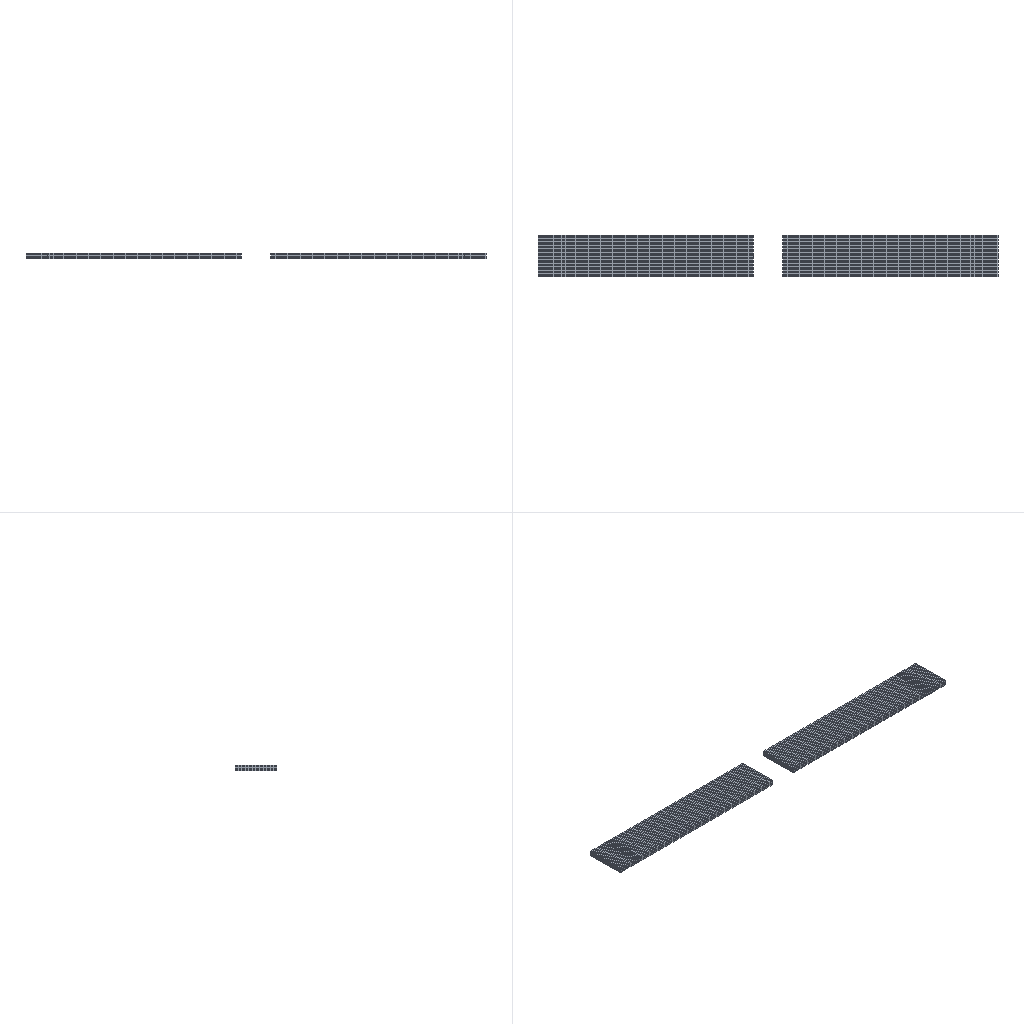Simulation study | abaqus
Set-up summary:
category,name,step,type,value,unit,region
solver,abaqus
solver,version,,,Abaqus/Standard 2020
units,not stated in the deck,,not stated
analysis,deck,,transient,transient
load_step,Step-1,Step-1,transient
load_step,requested,,,1
mesh,nodes,,,9920
mesh,elements,,,7200
element_type,C3D8R,,solid,7200
load,load commands in deck,,count,1
bc,support commands in deck,,count,6
material,MATERIAL-1,,in results
check,setup vs results,,match,"per instance, exact: element labels, types and connectivity; labels of the nodes the elements use; coordinates of those nodes at SINGLE_PRECISION in 1 of 4 instance(s)"
Abaqus input file, long lists of numbers shortened:
*Heading
** Job name: Job-1 Model name: Model-1
** Generated by: Abaqus/CAE 2020
*Preprint, echo=NO, model=NO, history=NO, contact=NO
**
** PARTS
**
*Part, name=Part-1
*Node
      1,           0.,           0.,           0.
      2,           0.,          -1.,           0.
** (4028 more lines like these left out)
*Element, type=C3D8R
   1,  156,  157,  188,  187,    1,    2,   33,   32
   2,  157,  158,  189,  188,    2,    3,   34,   33
** (2998 more lines like these left out)
*Nset, nset=Set-6, generate
    1,  4030,     1
*Elset, elset=Set-6, generate
    1,  3000,     1
** Section: Section-1
*Solid Section, elset=Set-6, material=Material-1
,
*End Part
**
*Part, name=Part-2
*Node
      1,           0.,         -30.,           4.
      2,           0.,         -29.,           4.
** (928 more lines like these left out)
*Element, type=C3D8R
  1, 156, 157, 188, 187,   1,   2,  33,  32
  2, 157, 158, 189, 188,   2,   3,  34,  33
** (598 more lines like these left out)
*Nset, nset=Set-7, generate
   1,  930,    1
*Elset, elset=Set-7, generate
   1,  600,    1
** Section: Section-1
*Solid Section, elset=Set-7, material=Material-1
,
*End Part
**
**
** ASSEMBLY
**
*Assembly, name=Assembly
**
*Instance, name=Part-1-1, part=Part-1
*End Instance
**
*Instance, name=Part-2-1, part=Part-2
       -15.5,           0.,           0.
*End Instance
**
*Instance, name=Part-1-1-rad-2, part=Part-1
        300.,         -30.,           0.
        300.,         -30.,           0.,         300.,         -30.,           1.,         180.
*End Instance
**
*Instance, name=Part-2-1-rad-2, part=Part-2
       315.5,         -30.,           0.
       315.5,         -30.,           0.,        315.5,         -30.,           1.,         180.
*End Instance
**
*Node
      1,         150.,         -15.,           2.
*Node
      2,         150.,         -15.,           3.
*Node
      3,         150.,         -15.,          2.5
*Node
      4,         150.,         -13.,          2.5
*Nset, nset=Set-2
 3,
*Nset, nset=Set-3, instance=Part-1-1
    1,   31,   94,  124,  125,  155,  931,  961, 1055, 1085, 3876, 3906, 4000, 4030
*Nset, nset=Set-3, instance=Part-2-1
   1,  31, 125, 155, 156, 186, 280, 310, 621, 651, 745, 775, 776, 806, 838, 868
 900, 930
*Nset, nset=Set-3, generate
 1,  3,  1
*Nset, nset=Set-3, instance=Part-1-1-rad-2
    1,   31,   94,  124,  125,  155,  931,  961, 1055, 1085, 3876, 3906, 4000, 4030
*Nset, nset=Set-3, instance=Part-2-1-rad-2
   1,  31, 125, 155, 156, 186, 280, 310, 621, 651, 745, 775, 776, 806, 838, 868
 900, 930
*Nset, nset=Set-4, instance=Part-1-1, generate
    1,  4030,     1
*Nset, nset=Set-4, instance=Part-2-1, generate
   1,  930,    1
*Nset, nset=Set-4, instance=Part-1-1-rad-2, generate
    1,  4030,     1
*Nset, nset=Set-4, instance=Part-2-1-rad-2, generate
   1,  930,    1
*Elset, elset=Set-4, instance=Part-1-1, generate
    1,  3000,     1
*Elset, elset=Set-4, instance=Part-2-1, generate
   1,  600,    1
*Elset, elset=Set-4, instance=Part-1-1-rad-2, generate
    1,  3000,     1
*Elset, elset=Set-4, instance=Part-2-1-rad-2, generate
   1,  600,    1
*Nset, nset=Set-5, instance=Part-1-1, generate
    1,  4030,     1
*Nset, nset=Set-5, instance=Part-2-1, generate
   1,  930,    1
*Nset, nset=Set-5, instance=Part-1-1-rad-2, generate
    1,  4030,     1
*Nset, nset=Set-5, instance=Part-2-1-rad-2, generate
   1,  930,    1
*Elset, elset=Set-5, instance=Part-1-1, generate
    1,  3000,     1
*Elset, elset=Set-5, instance=Part-2-1, generate
   1,  600,    1
*Elset, elset=Set-5, instance=Part-1-1-rad-2, generate
    1,  3000,     1
*Elset, elset=Set-5, instance=Part-2-1-rad-2, generate
   1,  600,    1
*Nset, nset=m_Set-1
 3,
*Elset, elset=_Surf-8_S5, internal, instance=Part-1-1
   91,   92,   93,   94,   95,   96,   97,   98,   99,  100,  101,  102,  103,  104,  105,  106
  107,  108,  109,  110,  111,  112,  113,  114,  115,  116,  117,  118,  119,  120,  211,  212
** (45 more lines like these left out)
*Elset, elset=_Surf-8_S5, internal, instance=Part-1-1-rad-2
   91,   92,   93,   94,   95,   96,   97,   98,   99,  100,  101,  102,  103,  104,  105,  106
  107,  108,  109,  110,  111,  112,  113,  114,  115,  116,  117,  118,  119,  120,  211,  212
** (45 more lines like these left out)
*Surface, type=ELEMENT, name=Surf-8
_Surf-8_S5, S5
*Elset, elset=_Surf-11_S5, internal, instance=Part-1-1
   91,   92,   93,   94,   95,   96,   97,   98,   99,  100,  101,  102,  103,  104,  105,  106
  107,  108,  109,  110,  111,  112,  113,  114,  115,  116,  117,  118,  119,  120,  211,  212
** (45 more lines like these left out)
*Elset, elset=_Surf-11_S5, internal, instance=Part-1-1-rad-2
   91,   92,   93,   94,   95,   96,   97,   98,   99,  100,  101,  102,  103,  104,  105,  106
  107,  108,  109,  110,  111,  112,  113,  114,  115,  116,  117,  118,  119,  120,  211,  212
** (45 more lines like these left out)
*Elset, elset=_Surf-11_S3, internal, instance=Part-2-1
   1,   2,   3,   4,   5,   6,   7,   8,   9,  10,  11,  12,  13,  14,  15,  16
  17,  18,  19,  20,  21,  22,  23,  24,  25,  26,  27,  28,  29,  30, 121, 122
** (8 more lines like these left out)
*Elset, elset=_Surf-11_S3, internal, instance=Part-2-1-rad-2
   1,   2,   3,   4,   5,   6,   7,   8,   9,  10,  11,  12,  13,  14,  15,  16
  17,  18,  19,  20,  21,  22,  23,  24,  25,  26,  27,  28,  29,  30, 121, 122
** (8 more lines like these left out)
*Surface, type=ELEMENT, name=Surf-11
_Surf-11_S5, S5
_Surf-11_S3, S3
*Elset, elset=_Surf-13_S5, internal, instance=Part-1-1
   91,   92,   93,   94,   95,   96,   97,   98,   99,  100,  101,  102,  103,  104,  105,  106
  107,  108,  109,  110,  111,  112,  113,  114,  115,  116,  117,  118,  119,  120,  211,  212
** (45 more lines like these left out)
*Elset, elset=_Surf-13_S5, internal, instance=Part-2-1
  91,  92,  93,  94,  95,  96,  97,  98,  99, 100, 101, 102, 103, 104, 105, 106
 107, 108, 109, 110, 111, 112, 113, 114, 115, 116, 117, 118, 119, 120, 211, 212
** (8 more lines like these left out)
*Elset, elset=_Surf-13_S5, internal, instance=Part-1-1-rad-2
   91,   92,   93,   94,   95,   96,   97,   98,   99,  100,  101,  102,  103,  104,  105,  106
  107,  108,  109,  110,  111,  112,  113,  114,  115,  116,  117,  118,  119,  120,  211,  212
** (45 more lines like these left out)
*Elset, elset=_Surf-13_S5, internal, instance=Part-2-1-rad-2
  91,  92,  93,  94,  95,  96,  97,  98,  99, 100, 101, 102, 103, 104, 105, 106
 107, 108, 109, 110, 111, 112, 113, 114, 115, 116, 117, 118, 119, 120, 211, 212
** (8 more lines like these left out)
*Elset, elset=_Surf-13_S4, internal, instance=Part-1-1, generate
   30,  3000,    30
*Elset, elset=_Surf-13_S4, internal, instance=Part-2-1, generate
  30,  600,   30
*Elset, elset=_Surf-13_S4, internal, instance=Part-1-1-rad-2, generate
   30,  3000,    30
*Elset, elset=_Surf-13_S4, internal, instance=Part-2-1-rad-2, generate
  30,  600,   30
*Elset, elset=_Surf-13_S3, internal, instance=Part-1-1
    1,    2,    3,    4,    5,    6,    7,    8,    9,   10,   11,   12,   13,   14,   15,   16
   17,   18,   19,   20,   21,   22,   23,   24,   25,   26,   27,   28,   29,   30,  121,  122
** (45 more lines like these left out)
*Elset, elset=_Surf-13_S3, internal, instance=Part-2-1
   1,   2,   3,   4,   5,   6,   7,   8,   9,  10,  11,  12,  13,  14,  15,  16
  17,  18,  19,  20,  21,  22,  23,  24,  25,  26,  27,  28,  29,  30, 121, 122
** (8 more lines like these left out)
*Elset, elset=_Surf-13_S3, internal, instance=Part-1-1-rad-2
    1,    2,    3,    4,    5,    6,    7,    8,    9,   10,   11,   12,   13,   14,   15,   16
   17,   18,   19,   20,   21,   22,   23,   24,   25,   26,   27,   28,   29,   30,  121,  122
** (45 more lines like these left out)
*Elset, elset=_Surf-13_S3, internal, instance=Part-2-1-rad-2
   1,   2,   3,   4,   5,   6,   7,   8,   9,  10,  11,  12,  13,  14,  15,  16
  17,  18,  19,  20,  21,  22,  23,  24,  25,  26,  27,  28,  29,  30, 121, 122
** (8 more lines like these left out)
*Elset, elset=_Surf-13_S6, internal, instance=Part-1-1, generate
    1,  2971,    30
*Elset, elset=_Surf-13_S6, internal, instance=Part-2-1, generate
   1,  571,   30
*Elset, elset=_Surf-13_S6, internal, instance=Part-1-1-rad-2, generate
    1,  2971,    30
*Elset, elset=_Surf-13_S6, internal, instance=Part-2-1-rad-2, generate
   1,  571,   30
*Elset, elset=_Surf-13_S2, internal, instance=Part-1-1, generate
   1,  120,    1
*Elset, elset=_Surf-13_S2, internal, instance=Part-2-1, generate
   1,  120,    1
*Elset, elset=_Surf-13_S2, internal, instance=Part-1-1-rad-2, generate
   1,  120,    1
*Elset, elset=_Surf-13_S2, internal, instance=Part-2-1-rad-2, generate
   1,  120,    1
*Elset, elset=_Surf-13_S1, internal, instance=Part-1-1, generate
 2881,  3000,     1
*Elset, elset=_Surf-13_S1, internal, instance=Part-2-1, generate
 481,  600,    1
*Elset, elset=_Surf-13_S1, internal, instance=Part-1-1-rad-2, generate
 2881,  3000,     1
*Elset, elset=_Surf-13_S1, internal, instance=Part-2-1-rad-2, generate
 481,  600,    1
*Surface, type=ELEMENT, name=Surf-13
_Surf-13_S5, S5
_Surf-13_S4, S4
_Surf-13_S6, S6
_Surf-13_S2, S2
_Surf-13_S3, S3
_Surf-13_S1, S1
*Elset, elset=_Surf-14_S2, internal, instance=Part-2-1, generate
   1,  120,    1
*Elset, elset=_Surf-14_S2, internal, instance=Part-2-1-rad-2, generate
   1,  120,    1
*Surface, type=ELEMENT, name=Surf-14
_Surf-14_S2, S2
*Elset, elset=_Surf-15_S5, internal, instance=Part-1-1
   91,   92,   93,   94,   95,   96,   97,   98,   99,  100,  101,  102,  103,  104,  105,  106
  107,  108,  109,  110,  111,  112,  113,  114,  115,  116,  117,  118,  119,  120,  211,  212
** (45 more lines like these left out)
*Elset, elset=_Surf-15_S5, internal, instance=Part-1-1-rad-2
   91,   92,   93,   94,   95,   96,   97,   98,   99,  100,  101,  102,  103,  104,  105,  106
  107,  108,  109,  110,  111,  112,  113,  114,  115,  116,  117,  118,  119,  120,  211,  212
** (45 more lines like these left out)
*Elset, elset=_Surf-15_S3, internal, instance=Part-2-1
   1,   2,   3,   4,   5,   6,   7,   8,   9,  10,  11,  12,  13,  14,  15,  16
  17,  18,  19,  20,  21,  22,  23,  24,  25,  26,  27,  28,  29,  30, 121, 122
** (8 more lines like these left out)
*Elset, elset=_Surf-15_S3, internal, instance=Part-2-1-rad-2
   1,   2,   3,   4,   5,   6,   7,   8,   9,  10,  11,  12,  13,  14,  15,  16
  17,  18,  19,  20,  21,  22,  23,  24,  25,  26,  27,  28,  29,  30, 121, 122
** (8 more lines like these left out)
*Surface, type=ELEMENT, name=Surf-15
_Surf-15_S5, S5
_Surf-15_S3, S3
*Elset, elset=_Surf-16_S5, internal, instance=Part-1-1
   91,   92,   93,   94,   95,   96,   97,   98,   99,  100,  101,  102,  103,  104,  105,  106
  107,  108,  109,  110,  111,  112,  113,  114,  115,  116,  117,  118,  119,  120,  211,  212
** (45 more lines like these left out)
*Elset, elset=_Surf-16_S5, internal, instance=Part-2-1-rad-2
  91,  92,  93,  94,  95,  96,  97,  98,  99, 100, 101, 102, 103, 104, 105, 106
 107, 108, 109, 110, 111, 112, 113, 114, 115, 116, 117, 118, 119, 120, 211, 212
** (8 more lines like these left out)
*Elset, elset=_Surf-16_S3, internal, instance=Part-2-1
   1,   2,   3,   4,   5,   6,   7,   8,   9,  10,  11,  12,  13,  14,  15,  16
  17,  18,  19,  20,  21,  22,  23,  24,  25,  26,  27,  28,  29,  30, 121, 122
** (8 more lines like these left out)
*Elset, elset=_Surf-16_S3, internal, instance=Part-1-1-rad-2
    1,    2,    3,    4,    5,    6,    7,    8,    9,   10,   11,   12,   13,   14,   15,   16
   17,   18,   19,   20,   21,   22,   23,   24,   25,   26,   27,   28,   29,   30,  121,  122
** (45 more lines like these left out)
*Surface, type=ELEMENT, name=Surf-16
_Surf-16_S5, S5
_Surf-16_S3, S3
*Elset, elset=_Surf-17_S3, internal, instance=Part-1-1
    1,    2,    3,    4,    5,    6,    7,    8,    9,   10,   11,   12,   13,   14,   15,   16
   17,   18,   19,   20,   21,   22,   23,   24,   25,   26,   27,   28,   29,   30,  121,  122
** (45 more lines like these left out)
*Elset, elset=_Surf-17_S3, internal, instance=Part-2-1-rad-2
   1,   2,   3,   4,   5,   6,   7,   8,   9,  10,  11,  12,  13,  14,  15,  16
  17,  18,  19,  20,  21,  22,  23,  24,  25,  26,  27,  28,  29,  30, 121, 122
** (8 more lines like these left out)
*Elset, elset=_Surf-17_S5, internal, instance=Part-2-1
  91,  92,  93,  94,  95,  96,  97,  98,  99, 100, 101, 102, 103, 104, 105, 106
 107, 108, 109, 110, 111, 112, 113, 114, 115, 116, 117, 118, 119, 120, 211, 212
** (8 more lines like these left out)
*Elset, elset=_Surf-17_S5, internal, instance=Part-1-1-rad-2
   91,   92,   93,   94,   95,   96,   97,   98,   99,  100,  101,  102,  103,  104,  105,  106
  107,  108,  109,  110,  111,  112,  113,  114,  115,  116,  117,  118,  119,  120,  211,  212
** (45 more lines like these left out)
*Surface, type=ELEMENT, name=Surf-17
_Surf-17_S3, S3
_Surf-17_S5, S5
*Elset, elset=_Surf-18_S5, internal, instance=Part-1-1
   91,   92,   93,   94,   95,   96,   97,   98,   99,  100,  101,  102,  103,  104,  105,  106
  107,  108,  109,  110,  111,  112,  113,  114,  115,  116,  117,  118,  119,  120,  211,  212
** (45 more lines like these left out)
*Elset, elset=_Surf-18_S5, internal, instance=Part-1-1-rad-2
   91,   92,   93,   94,   95,   96,   97,   98,   99,  100,  101,  102,  103,  104,  105,  106
  107,  108,  109,  110,  111,  112,  113,  114,  115,  116,  117,  118,  119,  120,  211,  212
** (45 more lines like these left out)
*Elset, elset=_Surf-18_S3, internal, instance=Part-2-1
   1,   2,   3,   4,   5,   6,   7,   8,   9,  10,  11,  12,  13,  14,  15,  16
  17,  18,  19,  20,  21,  22,  23,  24,  25,  26,  27,  28,  29,  30, 121, 122
** (8 more lines like these left out)
*Elset, elset=_Surf-18_S3, internal, instance=Part-2-1-rad-2
   1,   2,   3,   4,   5,   6,   7,   8,   9,  10,  11,  12,  13,  14,  15,  16
  17,  18,  19,  20,  21,  22,  23,  24,  25,  26,  27,  28,  29,  30, 121, 122
** (8 more lines like these left out)
*Surface, type=ELEMENT, name=Surf-18
_Surf-18_S5, S5
_Surf-18_S3, S3
*Elset, elset=_m_Surf-1_S2, internal, instance=Part-1-1, generate
  1,  90,   1
*Surface, type=ELEMENT, name=m_Surf-1
_m_Surf-1_S2, S2
*Elset, elset=_m_Surf-5_S2, internal, instance=Part-1-1-rad-2, generate
   1,  120,    1
*Surface, type=ELEMENT, name=m_Surf-5
_m_Surf-5_S2, S2
*Elset, elset=_s_Surf-3_S2, internal, instance=Part-1-1, generate
  91,  120,    1
*Surface, type=ELEMENT, name=s_Surf-3
_s_Surf-3_S2, S2
*Elset, elset=_s_Surf-7_S1, internal, instance=Part-1-1, generate
 2881,  3000,     1
*Elset, elset=_s_Surf-7_S1, internal, instance=Part-1-1-rad-2, generate
 2881,  3000,     1
*Surface, type=ELEMENT, name=s_Surf-7
_s_Surf-7_S1, S1
*Elset, elset=_s_Surf-9_S1, internal, instance=Part-2-1, generate
 541,  600,    1
*Surface, type=ELEMENT, name=s_Surf-9
_s_Surf-9_S1, S1
*Elset, elset=_s_Surf-10_S1, internal, instance=Part-2-1-rad-2, generate
 481,  600,    1
*Surface, type=ELEMENT, name=s_Surf-10
_s_Surf-10_S1, S1
*Elset, elset=_s_Surf-12_S1, internal, instance=Part-2-1, generate
 481,  540,    1
*Surface, type=ELEMENT, name=s_Surf-12
_s_Surf-12_S1, S1
** Constraint: Constraint-1
*Tie, name=Constraint-1, adjust=yes
s_Surf-9, m_Surf-1
** Constraint: Constraint-2
*Tie, name=Constraint-2, adjust=yes
s_Surf-10, m_Surf-5
** Constraint: Constraint-3
*Coupling, constraint name=Constraint-3, ref node=m_Set-1, surface=s_Surf-7
*Kinematic
*End Assembly
*Amplitude, name=Amp-1, definition=PERIODIC
1,           2093.,              0.,              0.
             1.,              0.
*Amplitude, name=Amp-2, definition=PERIODIC
1,            628.,              0.,              0.
             1.,              0.
**
** MATERIALS
**
*Material, name=Material-1
*Density
 7.8e-09,
*Elastic
210000., 0.3
**
** INTERACTION PROPERTIES
**
*Surface Interaction, name=IntProp-1
1.,
*Friction, slip tolerance=0.005
 0.2,
*Surface Behavior, pressure-overclosure=HARD
**
** INTERACTIONS
**
** Interaction: Int-1
*Contact Pair, interaction=IntProp-1, type=SURFACE TO SURFACE
s_Surf-12, s_Surf-3
** ----------------------------------------------------------------
**
** STEP: Step-1
**
*Step, name=Step-1, nlgeom=YES, inc=2000
*Dynamic,direct
3.5e-05,0.015,
**
** BOUNDARY CONDITIONS
**
** Name: BC-1 Type: 速度/角速度
*Boundary, type=VELOCITY
Set-2, 1, 1
Set-2, 2, 2
Set-2, 3, 3
Set-2, 4, 4
Set-2, 5, 5
Set-2, 6, 6
**
** LOADS
**
** Name: Load-3   Type: Rotational body force
*Dload
Set-5, CENTRIF, 4.38484e+06,150.,-13.,2.5,0.,-1.,0.
**
** OUTPUT REQUESTS
**
*Restart, write, number interval=1, time marks=NO
**
** FIELD OUTPUT: F-Output-1
**
*Output, field, frequency=1
*Node Output
A, RF, U, V
*Element Output, directions=YES
E, LE, MISES, PE, PEEQ, S
*Contact Output
CSTRESS,
**
** HISTORY OUTPUT: H-Output-1
**
*Output, history, variable=PRESELECT, number interval=200, time marks=NO
*End Step
Results summary:
result,step,,completed,increments=429 time=0.015/0.015
result,analysis,,,transient
result,last_loadstep,,,1
result,primary field,,,U
result,reaction total,,FX,0.2636,model units
result,reaction total,,FY,-0.0,model units
result,reaction total,,FZ,1385.849,model units